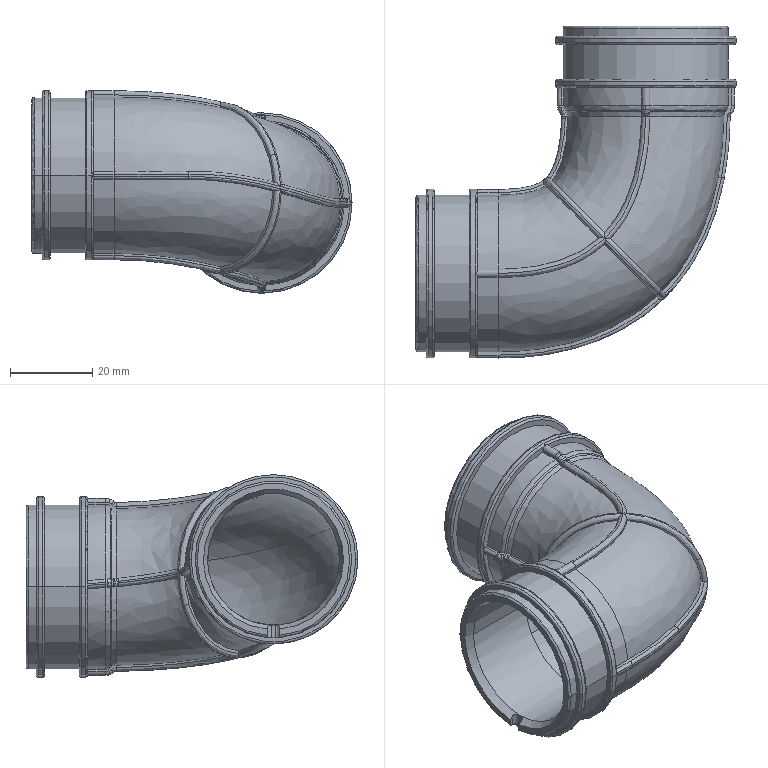Part | STEP file | ZXW722-L-91 | 1 solid | 262 faces | box 78.028 x 80.92 x 49.347 mm | volume 37026 mm3 | spline 153 | plane 43 | cylinder 40 | torus 21 | cone 3 | other 2 | commonest cylinder face diameters 38.2 x8 40.2 x8 1.4 x6 2 x6 41.2 x4 44 x4